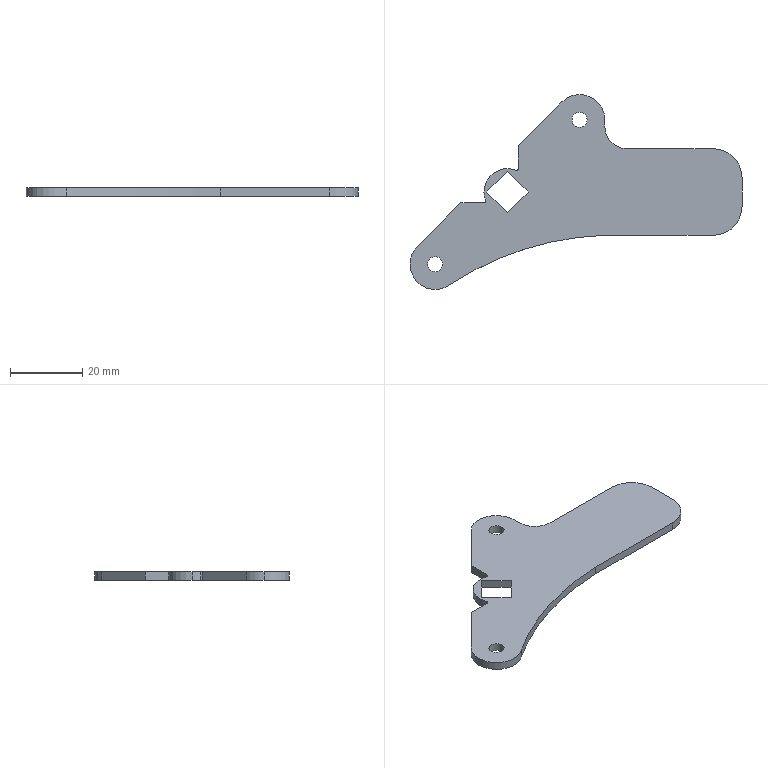Part | SolidWorks | features BaseBody 1 | 1 solid | 29 faces | box 92 x 54 x 2.3 mm | volume 5122 mm3 | cylinder 15 | plane 14 | commonest cylinder face diameters 4.2 x4 14 x3 1 x2 13 x2 16 x2 12 x1
STEP:
#1=CARTESIAN_POINT('',(-6.5,0.,2.3));
#2=VERTEX_POINT('',#1);
#3=CARTESIAN_POINT('',(-6.071,-2.321,2.3));
#4=VERTEX_POINT('',#3);
#5=CARTESIAN_POINT('',(0.,0.,2.3));
#6=DIRECTION('',(0.,0.,1.));
#7=DIRECTION('',(0.3571,0.934,0.));
#8=AXIS2_PLACEMENT_3D('',#5,#6,#7);
#9=CIRCLE('',#8,6.5);
#10=EDGE_CURVE('',#2,#4,#9,.T.);
#11=ORIENTED_EDGE('',*,*,#10,.F.);
#12=CARTESIAN_POINT('',(-6.5,0.,0.));
#13=VERTEX_POINT('',#12);
#14=CARTESIAN_POINT('',(-6.5,0.,2.3));
#15=DIRECTION('',(0.,0.,-1.));
#16=VECTOR('',#15,1000.);
#17=LINE('',#14,#16);
#18=EDGE_CURVE('',#2,#13,#17,.T.);
#19=ORIENTED_EDGE('',*,*,#18,.T.);
#20=CARTESIAN_POINT('',(-6.071,-2.321,0.));
#21=VERTEX_POINT('',#20);
#22=CARTESIAN_POINT('',(0.,0.,0.));
#23=DIRECTION('',(0.,0.,1.));
#24=DIRECTION('',(0.3571,0.934,0.));
#25=AXIS2_PLACEMENT_3D('',#22,#23,#24);
#26=CIRCLE('',#25,6.5);
#27=EDGE_CURVE('',#13,#21,#26,.T.);
#28=ORIENTED_EDGE('',*,*,#27,.T.);
#29=CARTESIAN_POINT('',(-6.071,-2.321,2.3));
#30=DIRECTION('',(0.,0.,-1.));
#31=VECTOR('',#30,1000.);
#32=LINE('',#29,#31);
#33=EDGE_CURVE('',#4,#21,#32,.T.);
#34=ORIENTED_EDGE('',*,*,#33,.F.);
#35=EDGE_LOOP('',(#11,#19,#28,#34));
#36=FACE_OUTER_BOUND('',#35,.T.);
#37=CARTESIAN_POINT('',(0.,0.,2.3));
#38=DIRECTION('',(0.,0.,-1.));
#39=DIRECTION('',(-1.,0.,0.));
#40=AXIS2_PLACEMENT_3D('',#37,#38,#39);
#41=CYLINDRICAL_SURFACE('',#40,6.5);
#42=ADVANCED_FACE('',(#36),#41,.T.);
#43=CARTESIAN_POINT('',(17.9,20.,2.3));
#44=VERTEX_POINT('',#43);
#45=CARTESIAN_POINT('',(22.1,20.,2.3));
#46=VERTEX_POINT('',#45);
#47=CARTESIAN_POINT('',(20.,20.,2.3));
#48=DIRECTION('',(0.,0.,1.));
#49=DIRECTION('',(1.,0.,0.));
#50=AXIS2_PLACEMENT_3D('',#47,#48,#49);
#51=CIRCLE('',#50,2.1);
#52=EDGE_CURVE('',#44,#46,#51,.T.);
#53=ORIENTED_EDGE('',*,*,#52,.T.);
#54=CARTESIAN_POINT('',(22.1,20.,0.));
#55=VERTEX_POINT('',#54);
#56=CARTESIAN_POINT('',(22.1,20.,2.3));
#57=DIRECTION('',(0.,0.,-1.));
#58=VECTOR('',#57,1000.);
#59=LINE('',#56,#58);
#60=EDGE_CURVE('',#46,#55,#59,.T.);
#61=ORIENTED_EDGE('',*,*,#60,.T.);
#62=CARTESIAN_POINT('',(17.9,20.,0.));
#63=VERTEX_POINT('',#62);
#64=CARTESIAN_POINT('',(20.,20.,0.));
#65=DIRECTION('',(0.,0.,1.));
#66=DIRECTION('',(1.,0.,0.));
#67=AXIS2_PLACEMENT_3D('',#64,#65,#66);
#68=CIRCLE('',#67,2.1);
#69=EDGE_CURVE('',#63,#55,#68,.T.);
#70=ORIENTED_EDGE('',*,*,#69,.F.);
#71=CARTESIAN_POINT('',(17.9,20.,2.3));
#72=DIRECTION('',(0.,0.,-1.));
#73=VECTOR('',#72,1000.);
#74=LINE('',#71,#73);
#75=EDGE_CURVE('',#44,#63,#74,.T.);
#76=ORIENTED_EDGE('',*,*,#75,.F.);
#77=EDGE_LOOP('',(#53,#61,#70,#76));
#78=FACE_OUTER_BOUND('',#77,.T.);
#79=CARTESIAN_POINT('',(20.,20.,2.3));
#80=DIRECTION('',(0.,0.,-1.));
#81=DIRECTION('',(-1.,0.,0.));
#82=AXIS2_PLACEMENT_3D('',#79,#80,#81);
#83=CYLINDRICAL_SURFACE('',#82,2.1);
#84=ADVANCED_FACE('',(#78),#83,.F.);
#85=CARTESIAN_POINT('',(-22.1,-20.,2.3));
#86=VERTEX_POINT('',#85);
#87=CARTESIAN_POINT('',(-17.9,-20.,2.3));
#88=VERTEX_POINT('',#87);
#89=CARTESIAN_POINT('',(-20.,-20.,2.3));
#90=DIRECTION('',(0.,0.,1.));
#91=DIRECTION('',(1.,0.,0.));
#92=AXIS2_PLACEMENT_3D('',#89,#90,#91);
#93=CIRCLE('',#92,2.1);
#94=EDGE_CURVE('',#86,#88,#93,.T.);
#95=ORIENTED_EDGE('',*,*,#94,.T.);
#96=CARTESIAN_POINT('',(-17.9,-20.,0.));
#97=VERTEX_POINT('',#96);
#98=CARTESIAN_POINT('',(-17.9,-20.,2.3));
#99=DIRECTION('',(0.,0.,-1.));
#100=VECTOR('',#99,1000.);
#101=LINE('',#98,#100);
#102=EDGE_CURVE('',#88,#97,#101,.T.);
#103=ORIENTED_EDGE('',*,*,#102,.T.);
#104=CARTESIAN_POINT('',(-22.1,-20.,0.));
#105=VERTEX_POINT('',#104);
#106=CARTESIAN_POINT('',(-20.,-20.,0.));
#107=DIRECTION('',(0.,0.,1.));
#108=DIRECTION('',(1.,0.,0.));
#109=AXIS2_PLACEMENT_3D('',#106,#107,#108);
#110=CIRCLE('',#109,2.1);
#111=EDGE_CURVE('',#105,#97,#110,.T.);
#112=ORIENTED_EDGE('',*,*,#111,.F.);
#113=CARTESIAN_POINT('',(-22.1,-20.,2.3));
#114=DIRECTION('',(0.,0.,-1.));
#115=VECTOR('',#114,1000.);
#116=LINE('',#113,#115);
#117=EDGE_CURVE('',#86,#105,#116,.T.);
#118=ORIENTED_EDGE('',*,*,#117,.F.);
#119=EDGE_LOOP('',(#95,#103,#112,#118));
#120=FACE_OUTER_BOUND('',#119,.T.);
#121=CARTESIAN_POINT('',(-20.,-20.,2.3));
#122=DIRECTION('',(0.,0.,-1.));
#123=DIRECTION('',(-1.,0.,0.));
#124=AXIS2_PLACEMENT_3D('',#121,#122,#123);
#125=CYLINDRICAL_SURFACE('',#124,2.1);
#126=ADVANCED_FACE('',(#120),#125,.F.);
#127=CARTESIAN_POINT('',(-27.,-20.,2.3));
#128=VERTEX_POINT('',#127);
#129=CARTESIAN_POINT('',(-15.783,-25.588,2.3));
#130=VERTEX_POINT('',#129);
#131=CARTESIAN_POINT('',(-20.,-20.,2.3));
#132=DIRECTION('',(0.,0.,1.));
#133=DIRECTION('',(-0.7071,0.7071,0.));
#134=AXIS2_PLACEMENT_3D('',#131,#132,#133);
#135=CIRCLE('',#134,7.);
#136=EDGE_CURVE('',#128,#130,#135,.T.);
#137=ORIENTED_EDGE('',*,*,#136,.F.);
#138=CARTESIAN_POINT('',(-27.,-20.,0.));
#139=VERTEX_POINT('',#138);
#140=CARTESIAN_POINT('',(-27.,-20.,2.3));
#141=DIRECTION('',(0.,0.,-1.));
#142=VECTOR('',#141,1000.);
#143=LINE('',#140,#142);
#144=EDGE_CURVE('',#128,#139,#143,.T.);
#145=ORIENTED_EDGE('',*,*,#144,.T.);
#146=CARTESIAN_POINT('',(-15.783,-25.588,0.));
#147=VERTEX_POINT('',#146);
#148=CARTESIAN_POINT('',(-20.,-20.,0.));
#149=DIRECTION('',(0.,0.,1.));
#150=DIRECTION('',(-0.7071,0.7071,0.));
#151=AXIS2_PLACEMENT_3D('',#148,#149,#150);
#152=CIRCLE('',#151,7.);
#153=EDGE_CURVE('',#139,#147,#152,.T.);
#154=ORIENTED_EDGE('',*,*,#153,.T.);
#155=CARTESIAN_POINT('',(-15.783,-25.588,2.3));
#156=DIRECTION('',(0.,0.,-1.));
#157=VECTOR('',#156,1000.);
#158=LINE('',#155,#157);
#159=EDGE_CURVE('',#130,#147,#158,.T.);
#160=ORIENTED_EDGE('',*,*,#159,.F.);
#161=EDGE_LOOP('',(#137,#145,#154,#160));
#162=FACE_OUTER_BOUND('',#161,.T.);
#163=CARTESIAN_POINT('',(-20.,-20.,2.3));
#164=DIRECTION('',(0.,0.,-1.));
#165=DIRECTION('',(-1.,0.,0.));
#166=AXIS2_PLACEMENT_3D('',#163,#164,#165);
#167=CYLINDRICAL_SURFACE('',#166,7.);
#168=ADVANCED_FACE('',(#162),#167,.T.);
#169=CARTESIAN_POINT('',(-12.899,-3.,0.));
#170=VERTEX_POINT('',#169);
#171=CARTESIAN_POINT('',(-24.95,-15.05,0.));
#172=VERTEX_POINT('',#171);
#173=CARTESIAN_POINT('',(-12.899,-3.,0.));
#174=DIRECTION('',(-0.7071,-0.7071,0.));
#175=VECTOR('',#174,1000.);
#176=LINE('',#173,#175);
#177=EDGE_CURVE('',#170,#172,#176,.T.);
#178=ORIENTED_EDGE('',*,*,#177,.T.);
#179=CARTESIAN_POINT('',(-24.95,-15.05,2.3));
#180=VERTEX_POINT('',#179);
#181=CARTESIAN_POINT('',(-24.95,-15.05,2.3));
#182=DIRECTION('',(0.,0.,-1.));
#183=VECTOR('',#182,1000.);
#184=LINE('',#181,#183);
#185=EDGE_CURVE('',#180,#172,#184,.T.);
#186=ORIENTED_EDGE('',*,*,#185,.F.);
#187=CARTESIAN_POINT('',(-12.899,-3.,2.3));
#188=VERTEX_POINT('',#187);
#189=CARTESIAN_POINT('',(-12.899,-3.,2.3));
#190=DIRECTION('',(-0.7071,-0.7071,0.));
#191=VECTOR('',#190,1000.);
#192=LINE('',#189,#191);
#193=EDGE_CURVE('',#188,#180,#192,.T.);
#194=ORIENTED_EDGE('',*,*,#193,.F.);
#195=CARTESIAN_POINT('',(-12.899,-3.,2.3));
#196=DIRECTION('',(0.,0.,-1.));
#197=VECTOR('',#196,1000.);
#198=LINE('',#195,#197);
#199=EDGE_CURVE('',#188,#170,#198,.T.);
#200=ORIENTED_EDGE('',*,*,#199,.T.);
#201=EDGE_LOOP('',(#178,#186,#194,#200));
#202=FACE_OUTER_BOUND('',#201,.T.);
#203=CARTESIAN_POINT('',(-12.899,-3.,2.3));
#204=DIRECTION('',(0.7071,-0.7071,0.));
#205=DIRECTION('',(0.7071,0.7071,0.));
#206=AXIS2_PLACEMENT_3D('',#203,#204,#205);
#207=PLANE('',#206);
#208=ADVANCED_FACE('',(#202),#207,.F.);
#209=ORIENTED_EDGE('',*,*,#111,.T.);
#210=CARTESIAN_POINT('',(-20.,-20.,0.));
#211=DIRECTION('',(0.,0.,1.));
#212=DIRECTION('',(1.,0.,0.));
#213=AXIS2_PLACEMENT_3D('',#210,#211,#212);
#214=CIRCLE('',#213,2.1);
#215=EDGE_CURVE('',#97,#105,#214,.T.);
#216=ORIENTED_EDGE('',*,*,#215,.T.);
#217=EDGE_LOOP('',(#209,#216));
#218=FACE_BOUND('',#217,.T.);
#219=CARTESIAN_POINT('',(0.,5.728,0.));
#220=VERTEX_POINT('',#219);
#221=CARTESIAN_POINT('',(-5.728,0.,0.));
#222=VERTEX_POINT('',#221);
#223=CARTESIAN_POINT('',(0.,5.728,0.));
#224=DIRECTION('',(-0.7071,-0.7071,0.));
#225=VECTOR('',#224,1000.);
#226=LINE('',#223,#225);
#227=EDGE_CURVE('',#220,#222,#226,.T.);
#228=ORIENTED_EDGE('',*,*,#227,.T.);
#229=CARTESIAN_POINT('',(0.,-5.728,0.));
#230=VERTEX_POINT('',#229);
#231=CARTESIAN_POINT('',(-5.728,0.,0.));
#232=DIRECTION('',(0.7071,-0.7071,0.));
#233=VECTOR('',#232,1000.);
#234=LINE('',#231,#233);
#235=EDGE_CURVE('',#222,#230,#234,.T.);
#236=ORIENTED_EDGE('',*,*,#235,.T.);
#237=CARTESIAN_POINT('',(5.728,0.,0.));
#238=VERTEX_POINT('',#237);
#239=CARTESIAN_POINT('',(0.,-5.728,0.));
#240=DIRECTION('',(0.7071,0.7071,0.));
#241=VECTOR('',#240,1000.);
#242=LINE('',#239,#241);
#243=EDGE_CURVE('',#230,#238,#242,.T.);
#244=ORIENTED_EDGE('',*,*,#243,.T.);
#245=CARTESIAN_POINT('',(5.728,0.,0.));
#246=DIRECTION('',(-0.7071,0.7071,0.));
#247=VECTOR('',#246,1000.);
#248=LINE('',#245,#247);
#249=EDGE_CURVE('',#238,#220,#248,.T.);
#250=ORIENTED_EDGE('',*,*,#249,.T.);
#251=EDGE_LOOP('',(#228,#236,#244,#250));
#252=FACE_BOUND('',#251,.T.);
#253=ORIENTED_EDGE('',*,*,#69,.T.);
#254=CARTESIAN_POINT('',(20.,20.,0.));
#255=DIRECTION('',(0.,0.,1.));
#256=DIRECTION('',(1.,0.,0.));
#257=AXIS2_PLACEMENT_3D('',#254,#255,#256);
#258=CIRCLE('',#257,2.1);
#259=EDGE_CURVE('',#55,#63,#258,.T.);
#260=ORIENTED_EDGE('',*,*,#259,.T.);
#261=EDGE_LOOP('',(#253,#260));
#262=FACE_BOUND('',#261,.T.);
#263=ORIENTED_EDGE('',*,*,#177,.F.);
#264=CARTESIAN_POINT('',(-6.538,-3.,0.));
#265=VERTEX_POINT('',#264);
#266=CARTESIAN_POINT('',(-6.538,-3.,0.));
#267=DIRECTION('',(-1.,0.,0.));
#268=VECTOR('',#267,1000.);
#269=LINE('',#266,#268);
#270=EDGE_CURVE('',#265,#170,#269,.T.);
#271=ORIENTED_EDGE('',*,*,#270,.F.);
#272=CARTESIAN_POINT('',(-6.538,-2.5,0.));
#273=DIRECTION('',(0.,0.,1.));
#274=DIRECTION('',(0.,-1.,0.));
#275=AXIS2_PLACEMENT_3D('',#272,#273,#274);
#276=CIRCLE('',#275,0.5);
#277=EDGE_CURVE('',#265,#21,#276,.T.);
#278=ORIENTED_EDGE('',*,*,#277,.T.);
#279=ORIENTED_EDGE('',*,*,#27,.F.);
#280=CARTESIAN_POINT('',(2.321,6.071,0.));
#281=VERTEX_POINT('',#280);
#282=CARTESIAN_POINT('',(0.,0.,0.));
#283=DIRECTION('',(0.,0.,1.));
#284=DIRECTION('',(0.3571,0.934,0.));
#285=AXIS2_PLACEMENT_3D('',#282,#283,#284);
#286=CIRCLE('',#285,6.5);
#287=EDGE_CURVE('',#281,#13,#286,.T.);
#288=ORIENTED_EDGE('',*,*,#287,.F.);
#289=CARTESIAN_POINT('',(3.,6.538,0.));
#290=VERTEX_POINT('',#289);
#291=CARTESIAN_POINT('',(2.5,6.538,0.));
#292=DIRECTION('',(0.,0.,1.));
#293=DIRECTION('',(-0.3571,-0.934,0.));
#294=AXIS2_PLACEMENT_3D('',#291,#292,#293);
#295=CIRCLE('',#294,0.5);
#296=EDGE_CURVE('',#281,#290,#295,.T.);
#297=ORIENTED_EDGE('',*,*,#296,.T.);
#298=CARTESIAN_POINT('',(3.,12.899,0.));
#299=VERTEX_POINT('',#298);
#300=CARTESIAN_POINT('',(3.,12.899,0.));
#301=DIRECTION('',(0.,-1.,0.));
#302=VECTOR('',#301,1000.);
#303=LINE('',#300,#302);
#304=EDGE_CURVE('',#299,#290,#303,.T.);
#305=ORIENTED_EDGE('',*,*,#304,.F.);
#306=CARTESIAN_POINT('',(15.05,24.95,0.));
#307=VERTEX_POINT('',#306);
#308=CARTESIAN_POINT('',(15.05,24.95,0.));
#309=DIRECTION('',(-0.7071,-0.7071,0.));
#310=VECTOR('',#309,1000.);
#311=LINE('',#308,#310);
#312=EDGE_CURVE('',#307,#299,#311,.T.);
#313=ORIENTED_EDGE('',*,*,#312,.F.);
#314=CARTESIAN_POINT('',(27.,20.,0.));
#315=VERTEX_POINT('',#314);
#316=CARTESIAN_POINT('',(20.,20.,0.));
#317=DIRECTION('',(0.,0.,1.));
#318=DIRECTION('',(1.,0.,0.));
#319=AXIS2_PLACEMENT_3D('',#316,#317,#318);
#320=CIRCLE('',#319,7.);
#321=EDGE_CURVE('',#315,#307,#320,.T.);
#322=ORIENTED_EDGE('',*,*,#321,.F.);
#323=CARTESIAN_POINT('',(27.,18.,0.));
#324=VERTEX_POINT('',#323);
#325=CARTESIAN_POINT('',(27.,18.,0.));
#326=DIRECTION('',(0.,1.,0.));
#327=VECTOR('',#326,1000.);
#328=LINE('',#325,#327);
#329=EDGE_CURVE('',#324,#315,#328,.T.);
#330=ORIENTED_EDGE('',*,*,#329,.F.);
#331=CARTESIAN_POINT('',(33.,12.,0.));
#332=VERTEX_POINT('',#331);
#333=CARTESIAN_POINT('',(33.,18.,0.));
#334=DIRECTION('',(0.,0.,1.));
#335=DIRECTION('',(-1.,0.,0.));
#336=AXIS2_PLACEMENT_3D('',#333,#334,#335);
#337=CIRCLE('',#336,6.);
#338=EDGE_CURVE('',#324,#332,#337,.T.);
#339=ORIENTED_EDGE('',*,*,#338,.T.);
#340=CARTESIAN_POINT('',(57.,12.,0.));
#341=VERTEX_POINT('',#340);
#342=CARTESIAN_POINT('',(57.,12.,0.));
#343=DIRECTION('',(-1.,0.,0.));
#344=VECTOR('',#343,1000.);
#345=LINE('',#342,#344);
#346=EDGE_CURVE('',#341,#332,#345,.T.);
#347=ORIENTED_EDGE('',*,*,#346,.F.);
#348=CARTESIAN_POINT('',(65.,4.,0.));
#349=VERTEX_POINT('',#348);
#350=CARTESIAN_POINT('',(57.,4.,0.));
#351=DIRECTION('',(0.,0.,1.));
#352=DIRECTION('',(1.,0.,0.));
#353=AXIS2_PLACEMENT_3D('',#350,#351,#352);
#354=CIRCLE('',#353,8.);
#355=EDGE_CURVE('',#349,#341,#354,.T.);
#356=ORIENTED_EDGE('',*,*,#355,.F.);
#357=CARTESIAN_POINT('',(65.,-4.,0.));
#358=VERTEX_POINT('',#357);
#359=CARTESIAN_POINT('',(65.,-4.,0.));
#360=DIRECTION('',(0.,1.,0.));
#361=VECTOR('',#360,1000.);
#362=LINE('',#359,#361);
#363=EDGE_CURVE('',#358,#349,#362,.T.);
#364=ORIENTED_EDGE('',*,*,#363,.F.);
#365=CARTESIAN_POINT('',(57.,-12.,0.));
#366=VERTEX_POINT('',#365);
#367=CARTESIAN_POINT('',(57.,-4.,0.));
#368=DIRECTION('',(0.,0.,1.));
#369=DIRECTION('',(0.,-1.,0.));
#370=AXIS2_PLACEMENT_3D('',#367,#368,#369);
#371=CIRCLE('',#370,8.);
#372=EDGE_CURVE('',#366,#358,#371,.T.);
#373=ORIENTED_EDGE('',*,*,#372,.F.);
#374=CARTESIAN_POINT('',(26.919,-12.,0.));
#375=VERTEX_POINT('',#374);
#376=CARTESIAN_POINT('',(26.919,-12.,0.));
#377=DIRECTION('',(1.,0.,0.));
#378=VECTOR('',#377,1000.);
#379=LINE('',#376,#378);
#380=EDGE_CURVE('',#375,#366,#379,.T.);
#381=ORIENTED_EDGE('',*,*,#380,.F.);
#382=CARTESIAN_POINT('',(29.8,-94.95,0.));
#383=DIRECTION('',(0.,0.,1.));
#384=DIRECTION('',(-0.03471,0.9994,0.));
#385=AXIS2_PLACEMENT_3D('',#382,#383,#384);
#386=CIRCLE('',#385,83.);
#387=EDGE_CURVE('',#375,#147,#386,.T.);
#388=ORIENTED_EDGE('',*,*,#387,.T.);
#389=ORIENTED_EDGE('',*,*,#153,.F.);
#390=CARTESIAN_POINT('',(-20.,-20.,0.));
#391=DIRECTION('',(0.,0.,1.));
#392=DIRECTION('',(-0.7071,0.7071,0.));
#393=AXIS2_PLACEMENT_3D('',#390,#391,#392);
#394=CIRCLE('',#393,7.);
#395=EDGE_CURVE('',#172,#139,#394,.T.);
#396=ORIENTED_EDGE('',*,*,#395,.F.);
#397=EDGE_LOOP('',(#263,#271,#278,#279,#288,#297,#305,#313,#322,#330,#339,#347,#356,#364,#373,#381,#388,#389,#396));
#398=FACE_OUTER_BOUND('',#397,.T.);
#399=CARTESIAN_POINT('',(-20.,-20.,0.));
#400=DIRECTION('',(0.,0.,1.));
#401=DIRECTION('',(1.,0.,0.));
#402=AXIS2_PLACEMENT_3D('',#399,#400,#401);
#403=PLANE('',#402);
#404=ADVANCED_FACE('',(#218,#252,#262,#398),#403,.F.);
#405=ORIENTED_EDGE('',*,*,#144,.F.);
#406=CARTESIAN_POINT('',(-20.,-20.,2.3));
#407=DIRECTION('',(0.,0.,1.));
#408=DIRECTION('',(-0.7071,0.7071,0.));
#409=AXIS2_PLACEMENT_3D('',#406,#407,#408);
#410=CIRCLE('',#409,7.);
#411=EDGE_CURVE('',#180,#128,#410,.T.);
#412=ORIENTED_EDGE('',*,*,#411,.F.);
#413=ORIENTED_EDGE('',*,*,#185,.T.);
#414=ORIENTED_EDGE('',*,*,#395,.T.);
#415=EDGE_LOOP('',(#405,#412,#413,#414));
#416=FACE_OUTER_BOUND('',#415,.T.);
#417=CARTESIAN_POINT('',(-20.,-20.,2.3));
#418=DIRECTION('',(0.,0.,-1.));
#419=DIRECTION('',(-1.,0.,0.));
#420=AXIS2_PLACEMENT_3D('',#417,#418,#419);
#421=CYLINDRICAL_SURFACE('',#420,7.);
#422=ADVANCED_FACE('',(#416),#421,.T.);
#423=ORIENTED_EDGE('',*,*,#94,.F.);
#424=CARTESIAN_POINT('',(-20.,-20.,2.3));
#425=DIRECTION('',(0.,0.,1.));
#426=DIRECTION('',(1.,0.,0.));
#427=AXIS2_PLACEMENT_3D('',#424,#425,#426);
#428=CIRCLE('',#427,2.1);
#429=EDGE_CURVE('',#88,#86,#428,.T.);
#430=ORIENTED_EDGE('',*,*,#429,.F.);
#431=EDGE_LOOP('',(#423,#430));
#432=FACE_BOUND('',#431,.T.);
#433=CARTESIAN_POINT('',(0.,5.728,2.3));
#434=VERTEX_POINT('',#433);
#435=CARTESIAN_POINT('',(-5.728,0.,2.3));
#436=VERTEX_POINT('',#435);
#437=CARTESIAN_POINT('',(0.,5.728,2.3));
#438=DIRECTION('',(-0.7071,-0.7071,0.));
#439=VECTOR('',#438,1000.);
#440=LINE('',#437,#439);
#441=EDGE_CURVE('',#434,#436,#440,.T.);
#442=ORIENTED_EDGE('',*,*,#441,.F.);
#443=CARTESIAN_POINT('',(5.728,0.,2.3));
#444=VERTEX_POINT('',#443);
#445=CARTESIAN_POINT('',(5.728,0.,2.3));
#446=DIRECTION('',(-0.7071,0.7071,0.));
#447=VECTOR('',#446,1000.);
#448=LINE('',#445,#447);
#449=EDGE_CURVE('',#444,#434,#448,.T.);
#450=ORIENTED_EDGE('',*,*,#449,.F.);
#451=CARTESIAN_POINT('',(0.,-5.728,2.3));
#452=VERTEX_POINT('',#451);
#453=CARTESIAN_POINT('',(0.,-5.728,2.3));
#454=DIRECTION('',(0.7071,0.7071,0.));
#455=VECTOR('',#454,1000.);
#456=LINE('',#453,#455);
#457=EDGE_CURVE('',#452,#444,#456,.T.);
#458=ORIENTED_EDGE('',*,*,#457,.F.);
#459=CARTESIAN_POINT('',(-5.728,0.,2.3));
#460=DIRECTION('',(0.7071,-0.7071,0.));
#461=VECTOR('',#460,1000.);
#462=LINE('',#459,#461);
#463=EDGE_CURVE('',#436,#452,#462,.T.);
#464=ORIENTED_EDGE('',*,*,#463,.F.);
#465=EDGE_LOOP('',(#442,#450,#458,#464));
#466=FACE_BOUND('',#465,.T.);
#467=ORIENTED_EDGE('',*,*,#52,.F.);
#468=CARTESIAN_POINT('',(20.,20.,2.3));
#469=DIRECTION('',(0.,0.,1.));
#470=DIRECTION('',(1.,0.,0.));
#471=AXIS2_PLACEMENT_3D('',#468,#469,#470);
#472=CIRCLE('',#471,2.1);
#473=EDGE_CURVE('',#46,#44,#472,.T.);
#474=ORIENTED_EDGE('',*,*,#473,.F.);
#475=EDGE_LOOP('',(#467,#474));
#476=FACE_BOUND('',#475,.T.);
#477=ORIENTED_EDGE('',*,*,#193,.T.);
#478=ORIENTED_EDGE('',*,*,#411,.T.);
#479=ORIENTED_EDGE('',*,*,#136,.T.);
#480=CARTESIAN_POINT('',(26.919,-12.,2.3));
#481=VERTEX_POINT('',#480);
#482=CARTESIAN_POINT('',(29.8,-94.95,2.3));
#483=DIRECTION('',(0.,0.,1.));
#484=DIRECTION('',(-0.03471,0.9994,0.));
#485=AXIS2_PLACEMENT_3D('',#482,#483,#484);
#486=CIRCLE('',#485,83.);
#487=EDGE_CURVE('',#481,#130,#486,.T.);
#488=ORIENTED_EDGE('',*,*,#487,.F.);
#489=CARTESIAN_POINT('',(57.,-12.,2.3));
#490=VERTEX_POINT('',#489);
#491=CARTESIAN_POINT('',(26.919,-12.,2.3));
#492=DIRECTION('',(1.,0.,0.));
#493=VECTOR('',#492,1000.);
#494=LINE('',#491,#493);
#495=EDGE_CURVE('',#481,#490,#494,.T.);
#496=ORIENTED_EDGE('',*,*,#495,.T.);
#497=CARTESIAN_POINT('',(65.,-4.,2.3));
#498=VERTEX_POINT('',#497);
#499=CARTESIAN_POINT('',(57.,-4.,2.3));
#500=DIRECTION('',(0.,0.,1.));
#501=DIRECTION('',(0.,-1.,0.));
#502=AXIS2_PLACEMENT_3D('',#499,#500,#501);
#503=CIRCLE('',#502,8.);
#504=EDGE_CURVE('',#490,#498,#503,.T.);
#505=ORIENTED_EDGE('',*,*,#504,.T.);
#506=CARTESIAN_POINT('',(65.,4.,2.3));
#507=VERTEX_POINT('',#506);
#508=CARTESIAN_POINT('',(65.,-4.,2.3));
#509=DIRECTION('',(0.,1.,0.));
#510=VECTOR('',#509,1000.);
#511=LINE('',#508,#510);
#512=EDGE_CURVE('',#498,#507,#511,.T.);
#513=ORIENTED_EDGE('',*,*,#512,.T.);
#514=CARTESIAN_POINT('',(57.,12.,2.3));
#515=VERTEX_POINT('',#514);
#516=CARTESIAN_POINT('',(57.,4.,2.3));
#517=DIRECTION('',(0.,0.,1.));
#518=DIRECTION('',(1.,0.,0.));
#519=AXIS2_PLACEMENT_3D('',#516,#517,#518);
#520=CIRCLE('',#519,8.);
#521=EDGE_CURVE('',#507,#515,#520,.T.);
#522=ORIENTED_EDGE('',*,*,#521,.T.);
#523=CARTESIAN_POINT('',(33.,12.,2.3));
#524=VERTEX_POINT('',#523);
#525=CARTESIAN_POINT('',(57.,12.,2.3));
#526=DIRECTION('',(-1.,0.,0.));
#527=VECTOR('',#526,1000.);
#528=LINE('',#525,#527);
#529=EDGE_CURVE('',#515,#524,#528,.T.);
#530=ORIENTED_EDGE('',*,*,#529,.T.);
#531=CARTESIAN_POINT('',(27.,18.,2.3));
#532=VERTEX_POINT('',#531);
#533=CARTESIAN_POINT('',(33.,18.,2.3));
#534=DIRECTION('',(0.,0.,1.));
#535=DIRECTION('',(-1.,0.,0.));
#536=AXIS2_PLACEMENT_3D('',#533,#534,#535);
#537=CIRCLE('',#536,6.);
#538=EDGE_CURVE('',#532,#524,#537,.T.);
#539=ORIENTED_EDGE('',*,*,#538,.F.);
#540=CARTESIAN_POINT('',(27.,20.,2.3));
#541=VERTEX_POINT('',#540);
#542=CARTESIAN_POINT('',(27.,18.,2.3));
#543=DIRECTION('',(0.,1.,0.));
#544=VECTOR('',#543,1000.);
#545=LINE('',#542,#544);
#546=EDGE_CURVE('',#532,#541,#545,.T.);
#547=ORIENTED_EDGE('',*,*,#546,.T.);
#548=CARTESIAN_POINT('',(15.05,24.95,2.3));
#549=VERTEX_POINT('',#548);
#550=CARTESIAN_POINT('',(20.,20.,2.3));
#551=DIRECTION('',(0.,0.,1.));
#552=DIRECTION('',(1.,0.,0.));
#553=AXIS2_PLACEMENT_3D('',#550,#551,#552);
#554=CIRCLE('',#553,7.);
#555=EDGE_CURVE('',#541,#549,#554,.T.);
#556=ORIENTED_EDGE('',*,*,#555,.T.);
#557=CARTESIAN_POINT('',(3.,12.899,2.3));
#558=VERTEX_POINT('',#557);
#559=CARTESIAN_POINT('',(15.05,24.95,2.3));
#560=DIRECTION('',(-0.7071,-0.7071,0.));
#561=VECTOR('',#560,1000.);
#562=LINE('',#559,#561);
#563=EDGE_CURVE('',#549,#558,#562,.T.);
#564=ORIENTED_EDGE('',*,*,#563,.T.);
#565=CARTESIAN_POINT('',(3.,6.538,2.3));
#566=VERTEX_POINT('',#565);
#567=CARTESIAN_POINT('',(3.,12.899,2.3));
#568=DIRECTION('',(0.,-1.,0.));
#569=VECTOR('',#568,1000.);
#570=LINE('',#567,#569);
#571=EDGE_CURVE('',#558,#566,#570,.T.);
#572=ORIENTED_EDGE('',*,*,#571,.T.);
#573=CARTESIAN_POINT('',(2.321,6.071,2.3));
#574=VERTEX_POINT('',#573);
#575=CARTESIAN_POINT('',(2.5,6.538,2.3));
#576=DIRECTION('',(0.,0.,1.));
#577=DIRECTION('',(-0.3571,-0.934,0.));
#578=AXIS2_PLACEMENT_3D('',#575,#576,#577);
#579=CIRCLE('',#578,0.5);
#580=EDGE_CURVE('',#574,#566,#579,.T.);
#581=ORIENTED_EDGE('',*,*,#580,.F.);
#582=CARTESIAN_POINT('',(0.,0.,2.3));
#583=DIRECTION('',(0.,0.,1.));
#584=DIRECTION('',(0.3571,0.934,0.));
#585=AXIS2_PLACEMENT_3D('',#582,#583,#584);
#586=CIRCLE('',#585,6.5);
#587=EDGE_CURVE('',#574,#2,#586,.T.);
#588=ORIENTED_EDGE('',*,*,#587,.T.);
#589=ORIENTED_EDGE('',*,*,#10,.T.);
#590=CARTESIAN_POINT('',(-6.538,-3.,2.3));
#591=VERTEX_POINT('',#590);
#592=CARTESIAN_POINT('',(-6.538,-2.5,2.3));
#593=DIRECTION('',(0.,0.,1.));
#594=DIRECTION('',(0.,-1.,0.));
#595=AXIS2_PLACEMENT_3D('',#592,#593,#594);
#596=CIRCLE('',#595,0.5);
#597=EDGE_CURVE('',#591,#4,#596,.T.);
#598=ORIENTED_EDGE('',*,*,#597,.F.);
#599=CARTESIAN_POINT('',(-6.538,-3.,2.3));
#600=DIRECTION('',(-1.,0.,0.));
#601=VECTOR('',#600,1000.);
#602=LINE('',#599,#601);
#603=EDGE_CURVE('',#591,#188,#602,.T.);
#604=ORIENTED_EDGE('',*,*,#603,.T.);
#605=EDGE_LOOP('',(#477,#478,#479,#488,#496,#505,#513,#522,#530,#539,#547,#556,#564,#572,#581,#588,#589,#598,#604));
#606=FACE_OUTER_BOUND('',#605,.T.);
#607=CARTESIAN_POINT('',(-20.,-20.,2.3));
#608=DIRECTION('',(0.,0.,1.));
#609=DIRECTION('',(1.,0.,0.));
#610=AXIS2_PLACEMENT_3D('',#607,#608,#609);
#611=PLANE('',#610);
#612=ADVANCED_FACE('',(#432,#466,#476,#606),#611,.T.);
#613=ORIENTED_EDGE('',*,*,#270,.T.);
#614=ORIENTED_EDGE('',*,*,#199,.F.);
#615=ORIENTED_EDGE('',*,*,#603,.F.);
#616=CARTESIAN_POINT('',(-6.538,-3.,2.3));
#617=DIRECTION('',(0.,0.,-1.));
#618=VECTOR('',#617,1000.);
#619=LINE('',#616,#618);
#620=EDGE_CURVE('',#591,#265,#619,.T.);
#621=ORIENTED_EDGE('',*,*,#620,.T.);
#622=EDGE_LOOP('',(#613,#614,#615,#621));
#623=FACE_OUTER_BOUND('',#622,.T.);
#624=CARTESIAN_POINT('',(-6.538,-3.,2.3));
#625=DIRECTION('',(0.,-1.,0.));
#626=DIRECTION('',(0.,0.,-1.));
#627=AXIS2_PLACEMENT_3D('',#624,#625,#626);
#628=PLANE('',#627);
#629=ADVANCED_FACE('',(#623),#628,.F.);
#630=ORIENTED_EDGE('',*,*,#102,.F.);
#631=ORIENTED_EDGE('',*,*,#429,.T.);
#632=ORIENTED_EDGE('',*,*,#117,.T.);
#633=ORIENTED_EDGE('',*,*,#215,.F.);
#634=EDGE_LOOP('',(#630,#631,#632,#633));
#635=FACE_OUTER_BOUND('',#634,.T.);
#636=CARTESIAN_POINT('',(-20.,-20.,2.3));
#637=DIRECTION('',(0.,0.,-1.));
#638=DIRECTION('',(-1.,0.,0.));
#639=AXIS2_PLACEMENT_3D('',#636,#637,#638);
#640=CYLINDRICAL_SURFACE('',#639,2.1);
#641=ADVANCED_FACE('',(#635),#640,.F.);
#642=ORIENTED_EDGE('',*,*,#227,.F.);
#643=CARTESIAN_POINT('',(0.,5.728,2.3));
#644=DIRECTION('',(0.,0.,-1.));
#645=VECTOR('',#644,1000.);
#646=LINE('',#643,#645);
#647=EDGE_CURVE('',#434,#220,#646,.T.);
#648=ORIENTED_EDGE('',*,*,#647,.F.);
#649=ORIENTED_EDGE('',*,*,#441,.T.);
#650=CARTESIAN_POINT('',(-5.728,0.,2.3));
#651=DIRECTION('',(0.,0.,-1.));
#652=VECTOR('',#651,1000.);
#653=LINE('',#650,#652);
#654=EDGE_CURVE('',#436,#222,#653,.T.);
#655=ORIENTED_EDGE('',*,*,#654,.T.);
#656=EDGE_LOOP('',(#642,#648,#649,#655));
#657=FACE_OUTER_BOUND('',#656,.T.);
#658=CARTESIAN_POINT('',(0.,5.728,2.3));
#659=DIRECTION('',(0.7071,-0.7071,0.));
#660=DIRECTION('',(0.7071,0.7071,0.));
#661=AXIS2_PLACEMENT_3D('',#658,#659,#660);
#662=PLANE('',#661);
#663=ADVANCED_FACE('',(#657),#662,.T.);
#664=ORIENTED_EDGE('',*,*,#235,.F.);
#665=ORIENTED_EDGE('',*,*,#654,.F.);
#666=ORIENTED_EDGE('',*,*,#463,.T.);
#667=CARTESIAN_POINT('',(0.,-5.728,2.3));
#668=DIRECTION('',(0.,0.,-1.));
#669=VECTOR('',#668,1000.);
#670=LINE('',#667,#669);
#671=EDGE_CURVE('',#452,#230,#670,.T.);
#672=ORIENTED_EDGE('',*,*,#671,.T.);
#673=EDGE_LOOP('',(#664,#665,#666,#672));
#674=FACE_OUTER_BOUND('',#673,.T.);
#675=CARTESIAN_POINT('',(-5.728,0.,2.3));
#676=DIRECTION('',(0.7071,0.7071,0.));
#677=DIRECTION('',(-0.7071,0.7071,0.));
#678=AXIS2_PLACEMENT_3D('',#675,#676,#677);
#679=PLANE('',#678);
#680=ADVANCED_FACE('',(#674),#679,.T.);
#681=ORIENTED_EDGE('',*,*,#243,.F.);
#682=ORIENTED_EDGE('',*,*,#671,.F.);
#683=ORIENTED_EDGE('',*,*,#457,.T.);
#684=CARTESIAN_POINT('',(5.728,0.,2.3));
#685=DIRECTION('',(0.,0.,-1.));
#686=VECTOR('',#685,1000.);
#687=LINE('',#684,#686);
#688=EDGE_CURVE('',#444,#238,#687,.T.);
#689=ORIENTED_EDGE('',*,*,#688,.T.);
#690=EDGE_LOOP('',(#681,#682,#683,#689));
#691=FACE_OUTER_BOUND('',#690,.T.);
#692=CARTESIAN_POINT('',(0.,-5.728,2.3));
#693=DIRECTION('',(-0.7071,0.7071,0.));
#694=DIRECTION('',(-0.7071,-0.7071,0.));
#695=AXIS2_PLACEMENT_3D('',#692,#693,#694);
#696=PLANE('',#695);
#697=ADVANCED_FACE('',(#691),#696,.T.);
#698=ORIENTED_EDGE('',*,*,#249,.F.);
#699=ORIENTED_EDGE('',*,*,#688,.F.);
#700=ORIENTED_EDGE('',*,*,#449,.T.);
#701=ORIENTED_EDGE('',*,*,#647,.T.);
#702=EDGE_LOOP('',(#698,#699,#700,#701));
#703=FACE_OUTER_BOUND('',#702,.T.);
#704=CARTESIAN_POINT('',(5.728,0.,2.3));
#705=DIRECTION('',(-0.7071,-0.7071,0.));
#706=DIRECTION('',(0.7071,-0.7071,0.));
#707=AXIS2_PLACEMENT_3D('',#704,#705,#706);
#708=PLANE('',#707);
#709=ADVANCED_FACE('',(#703),#708,.T.);
#710=ORIENTED_EDGE('',*,*,#60,.F.);
#711=ORIENTED_EDGE('',*,*,#473,.T.);
#712=ORIENTED_EDGE('',*,*,#75,.T.);
#713=ORIENTED_EDGE('',*,*,#259,.F.);
#714=EDGE_LOOP('',(#710,#711,#712,#713));
#715=FACE_OUTER_BOUND('',#714,.T.);
#716=CARTESIAN_POINT('',(20.,20.,2.3));
#717=DIRECTION('',(0.,0.,-1.));
#718=DIRECTION('',(-1.,0.,0.));
#719=AXIS2_PLACEMENT_3D('',#716,#717,#718);
#720=CYLINDRICAL_SURFACE('',#719,2.1);
#721=ADVANCED_FACE('',(#715),#720,.F.);
#722=ORIENTED_EDGE('',*,*,#277,.F.);
#723=ORIENTED_EDGE('',*,*,#620,.F.);
#724=ORIENTED_EDGE('',*,*,#597,.T.);
#725=ORIENTED_EDGE('',*,*,#33,.T.);
#726=EDGE_LOOP('',(#722,#723,#724,#725));
#727=FACE_OUTER_BOUND('',#726,.T.);
#728=CARTESIAN_POINT('',(-6.538,-2.5,2.3));
#729=DIRECTION('',(0.,0.,-1.));
#730=DIRECTION('',(-1.,0.,0.));
#731=AXIS2_PLACEMENT_3D('',#728,#729,#730);
#732=CYLINDRICAL_SURFACE('',#731,0.5);
#733=ADVANCED_FACE('',(#727),#732,.F.);
#734=ORIENTED_EDGE('',*,*,#18,.F.);
#735=ORIENTED_EDGE('',*,*,#587,.F.);
#736=CARTESIAN_POINT('',(2.321,6.071,2.3));
#737=DIRECTION('',(0.,0.,-1.));
#738=VECTOR('',#737,1000.);
#739=LINE('',#736,#738);
#740=EDGE_CURVE('',#574,#281,#739,.T.);
#741=ORIENTED_EDGE('',*,*,#740,.T.);
#742=ORIENTED_EDGE('',*,*,#287,.T.);
#743=EDGE_LOOP('',(#734,#735,#741,#742));
#744=FACE_OUTER_BOUND('',#743,.T.);
#745=CARTESIAN_POINT('',(0.,0.,2.3));
#746=DIRECTION('',(0.,0.,-1.));
#747=DIRECTION('',(-1.,0.,0.));
#748=AXIS2_PLACEMENT_3D('',#745,#746,#747);
#749=CYLINDRICAL_SURFACE('',#748,6.5);
#750=ADVANCED_FACE('',(#744),#749,.T.);
#751=ORIENTED_EDGE('',*,*,#296,.F.);
#752=ORIENTED_EDGE('',*,*,#740,.F.);
#753=ORIENTED_EDGE('',*,*,#580,.T.);
#754=CARTESIAN_POINT('',(3.,6.538,2.3));
#755=DIRECTION('',(0.,0.,-1.));
#756=VECTOR('',#755,1000.);
#757=LINE('',#754,#756);
#758=EDGE_CURVE('',#566,#290,#757,.T.);
#759=ORIENTED_EDGE('',*,*,#758,.T.);
#760=EDGE_LOOP('',(#751,#752,#753,#759));
#761=FACE_OUTER_BOUND('',#760,.T.);
#762=CARTESIAN_POINT('',(2.5,6.538,2.3));
#763=DIRECTION('',(0.,0.,-1.));
#764=DIRECTION('',(-1.,0.,0.));
#765=AXIS2_PLACEMENT_3D('',#762,#763,#764);
#766=CYLINDRICAL_SURFACE('',#765,0.5);
#767=ADVANCED_FACE('',(#761),#766,.F.);
#768=ORIENTED_EDGE('',*,*,#304,.T.);
#769=ORIENTED_EDGE('',*,*,#758,.F.);
#770=ORIENTED_EDGE('',*,*,#571,.F.);
#771=CARTESIAN_POINT('',(3.,12.899,2.3));
#772=DIRECTION('',(0.,0.,-1.));
#773=VECTOR('',#772,1000.);
#774=LINE('',#771,#773);
#775=EDGE_CURVE('',#558,#299,#774,.T.);
#776=ORIENTED_EDGE('',*,*,#775,.T.);
#777=EDGE_LOOP('',(#768,#769,#770,#776));
#778=FACE_OUTER_BOUND('',#777,.T.);
#779=CARTESIAN_POINT('',(3.,12.899,2.3));
#780=DIRECTION('',(1.,0.,0.));
#781=DIRECTION('',(0.,0.,-1.));
#782=AXIS2_PLACEMENT_3D('',#779,#780,#781);
#783=PLANE('',#782);
#784=ADVANCED_FACE('',(#778),#783,.F.);
#785=ORIENTED_EDGE('',*,*,#312,.T.);
#786=ORIENTED_EDGE('',*,*,#775,.F.);
#787=ORIENTED_EDGE('',*,*,#563,.F.);
#788=CARTESIAN_POINT('',(15.05,24.95,2.3));
#789=DIRECTION('',(0.,0.,-1.));
#790=VECTOR('',#789,1000.);
#791=LINE('',#788,#790);
#792=EDGE_CURVE('',#549,#307,#791,.T.);
#793=ORIENTED_EDGE('',*,*,#792,.T.);
#794=EDGE_LOOP('',(#785,#786,#787,#793));
#795=FACE_OUTER_BOUND('',#794,.T.);
#796=CARTESIAN_POINT('',(15.05,24.95,2.3));
#797=DIRECTION('',(0.7071,-0.7071,0.));
#798=DIRECTION('',(0.7071,0.7071,0.));
#799=AXIS2_PLACEMENT_3D('',#796,#797,#798);
#800=PLANE('',#799);
#801=ADVANCED_FACE('',(#795),#800,.F.);
#802=ORIENTED_EDGE('',*,*,#321,.T.);
#803=ORIENTED_EDGE('',*,*,#792,.F.);
#804=ORIENTED_EDGE('',*,*,#555,.F.);
#805=CARTESIAN_POINT('',(27.,20.,2.3));
#806=DIRECTION('',(0.,0.,-1.));
#807=VECTOR('',#806,1000.);
#808=LINE('',#805,#807);
#809=EDGE_CURVE('',#541,#315,#808,.T.);
#810=ORIENTED_EDGE('',*,*,#809,.T.);
#811=EDGE_LOOP('',(#802,#803,#804,#810));
#812=FACE_OUTER_BOUND('',#811,.T.);
#813=CARTESIAN_POINT('',(20.,20.,2.3));
#814=DIRECTION('',(0.,0.,-1.));
#815=DIRECTION('',(-1.,0.,0.));
#816=AXIS2_PLACEMENT_3D('',#813,#814,#815);
#817=CYLINDRICAL_SURFACE('',#816,7.);
#818=ADVANCED_FACE('',(#812),#817,.T.);
#819=ORIENTED_EDGE('',*,*,#329,.T.);
#820=ORIENTED_EDGE('',*,*,#809,.F.);
#821=ORIENTED_EDGE('',*,*,#546,.F.);
#822=CARTESIAN_POINT('',(27.,18.,2.3));
#823=DIRECTION('',(0.,0.,-1.));
#824=VECTOR('',#823,1000.);
#825=LINE('',#822,#824);
#826=EDGE_CURVE('',#532,#324,#825,.T.);
#827=ORIENTED_EDGE('',*,*,#826,.T.);
#828=EDGE_LOOP('',(#819,#820,#821,#827));
#829=FACE_OUTER_BOUND('',#828,.T.);
#830=CARTESIAN_POINT('',(27.,18.,2.3));
#831=DIRECTION('',(-1.,0.,0.));
#832=DIRECTION('',(0.,0.,1.));
#833=AXIS2_PLACEMENT_3D('',#830,#831,#832);
#834=PLANE('',#833);
#835=ADVANCED_FACE('',(#829),#834,.F.);
#836=ORIENTED_EDGE('',*,*,#338,.F.);
#837=ORIENTED_EDGE('',*,*,#826,.F.);
#838=ORIENTED_EDGE('',*,*,#538,.T.);
#839=CARTESIAN_POINT('',(33.,12.,2.3));
#840=DIRECTION('',(0.,0.,-1.));
#841=VECTOR('',#840,1000.);
#842=LINE('',#839,#841);
#843=EDGE_CURVE('',#524,#332,#842,.T.);
#844=ORIENTED_EDGE('',*,*,#843,.T.);
#845=EDGE_LOOP('',(#836,#837,#838,#844));
#846=FACE_OUTER_BOUND('',#845,.T.);
#847=CARTESIAN_POINT('',(33.,18.,2.3));
#848=DIRECTION('',(0.,0.,-1.));
#849=DIRECTION('',(-1.,0.,0.));
#850=AXIS2_PLACEMENT_3D('',#847,#848,#849);
#851=CYLINDRICAL_SURFACE('',#850,6.);
#852=ADVANCED_FACE('',(#846),#851,.F.);
#853=ORIENTED_EDGE('',*,*,#346,.T.);
#854=ORIENTED_EDGE('',*,*,#843,.F.);
#855=ORIENTED_EDGE('',*,*,#529,.F.);
#856=CARTESIAN_POINT('',(57.,12.,2.3));
#857=DIRECTION('',(0.,0.,-1.));
#858=VECTOR('',#857,1000.);
#859=LINE('',#856,#858);
#860=EDGE_CURVE('',#515,#341,#859,.T.);
#861=ORIENTED_EDGE('',*,*,#860,.T.);
#862=EDGE_LOOP('',(#853,#854,#855,#861));
#863=FACE_OUTER_BOUND('',#862,.T.);
#864=CARTESIAN_POINT('',(57.,12.,2.3));
#865=DIRECTION('',(0.,-1.,0.));
#866=DIRECTION('',(0.,0.,-1.));
#867=AXIS2_PLACEMENT_3D('',#864,#865,#866);
#868=PLANE('',#867);
#869=ADVANCED_FACE('',(#863),#868,.F.);
#870=ORIENTED_EDGE('',*,*,#355,.T.);
#871=ORIENTED_EDGE('',*,*,#860,.F.);
#872=ORIENTED_EDGE('',*,*,#521,.F.);
#873=CARTESIAN_POINT('',(65.,4.,2.3));
#874=DIRECTION('',(0.,0.,-1.));
#875=VECTOR('',#874,1000.);
#876=LINE('',#873,#875);
#877=EDGE_CURVE('',#507,#349,#876,.T.);
#878=ORIENTED_EDGE('',*,*,#877,.T.);
#879=EDGE_LOOP('',(#870,#871,#872,#878));
#880=FACE_OUTER_BOUND('',#879,.T.);
#881=CARTESIAN_POINT('',(57.,4.,2.3));
#882=DIRECTION('',(0.,0.,-1.));
#883=DIRECTION('',(-1.,0.,0.));
#884=AXIS2_PLACEMENT_3D('',#881,#882,#883);
#885=CYLINDRICAL_SURFACE('',#884,8.);
#886=ADVANCED_FACE('',(#880),#885,.T.);
#887=ORIENTED_EDGE('',*,*,#363,.T.);
#888=ORIENTED_EDGE('',*,*,#877,.F.);
#889=ORIENTED_EDGE('',*,*,#512,.F.);
#890=CARTESIAN_POINT('',(65.,-4.,2.3));
#891=DIRECTION('',(0.,0.,-1.));
#892=VECTOR('',#891,1000.);
#893=LINE('',#890,#892);
#894=EDGE_CURVE('',#498,#358,#893,.T.);
#895=ORIENTED_EDGE('',*,*,#894,.T.);
#896=EDGE_LOOP('',(#887,#888,#889,#895));
#897=FACE_OUTER_BOUND('',#896,.T.);
#898=CARTESIAN_POINT('',(65.,-4.,2.3));
#899=DIRECTION('',(-1.,0.,0.));
#900=DIRECTION('',(0.,0.,1.));
#901=AXIS2_PLACEMENT_3D('',#898,#899,#900);
#902=PLANE('',#901);
#903=ADVANCED_FACE('',(#897),#902,.F.);
#904=ORIENTED_EDGE('',*,*,#372,.T.);
#905=ORIENTED_EDGE('',*,*,#894,.F.);
#906=ORIENTED_EDGE('',*,*,#504,.F.);
#907=CARTESIAN_POINT('',(57.,-12.,2.3));
#908=DIRECTION('',(0.,0.,-1.));
#909=VECTOR('',#908,1000.);
#910=LINE('',#907,#909);
#911=EDGE_CURVE('',#490,#366,#910,.T.);
#912=ORIENTED_EDGE('',*,*,#911,.T.);
#913=EDGE_LOOP('',(#904,#905,#906,#912));
#914=FACE_OUTER_BOUND('',#913,.T.);
#915=CARTESIAN_POINT('',(57.,-4.,2.3));
#916=DIRECTION('',(0.,0.,-1.));
#917=DIRECTION('',(-1.,0.,0.));
#918=AXIS2_PLACEMENT_3D('',#915,#916,#917);
#919=CYLINDRICAL_SURFACE('',#918,8.);
#920=ADVANCED_FACE('',(#914),#919,.T.);
#921=ORIENTED_EDGE('',*,*,#380,.T.);
#922=ORIENTED_EDGE('',*,*,#911,.F.);
#923=ORIENTED_EDGE('',*,*,#495,.F.);
#924=CARTESIAN_POINT('',(26.919,-12.,2.3));
#925=DIRECTION('',(0.,0.,-1.));
#926=VECTOR('',#925,1000.);
#927=LINE('',#924,#926);
#928=EDGE_CURVE('',#481,#375,#927,.T.);
#929=ORIENTED_EDGE('',*,*,#928,.T.);
#930=EDGE_LOOP('',(#921,#922,#923,#929));
#931=FACE_OUTER_BOUND('',#930,.T.);
#932=CARTESIAN_POINT('',(26.919,-12.,2.3));
#933=DIRECTION('',(0.,1.,0.));
#934=DIRECTION('',(0.,0.,1.));
#935=AXIS2_PLACEMENT_3D('',#932,#933,#934);
#936=PLANE('',#935);
#937=ADVANCED_FACE('',(#931),#936,.F.);
#938=ORIENTED_EDGE('',*,*,#387,.F.);
#939=ORIENTED_EDGE('',*,*,#928,.F.);
#940=ORIENTED_EDGE('',*,*,#487,.T.);
#941=ORIENTED_EDGE('',*,*,#159,.T.);
#942=EDGE_LOOP('',(#938,#939,#940,#941));
#943=FACE_OUTER_BOUND('',#942,.T.);
#944=CARTESIAN_POINT('',(29.8,-94.95,2.3));
#945=DIRECTION('',(0.,0.,-1.));
#946=DIRECTION('',(-1.,0.,0.));
#947=AXIS2_PLACEMENT_3D('',#944,#945,#946);
#948=CYLINDRICAL_SURFACE('',#947,83.);
#949=ADVANCED_FACE('',(#943),#948,.F.);
#950=CLOSED_SHELL('',(#42,#84,#126,#168,#208,#404,#422,#612,#629,#641,#663,#680,#697,#709,#721,#733,#750,#767,#784,#801,#818,#835,#852,#869,#886,#903,#920,#937,#949));
#951=MANIFOLD_SOLID_BREP('',#950);
#952=CARTESIAN_POINT('',(0.,0.,0.));
#953=DIRECTION('',(0.,0.,1.));
#954=DIRECTION('',(1.,0.,0.));
#955=AXIS2_PLACEMENT_3D('',#952,#953,#954);
#956=(LENGTH_UNIT()NAMED_UNIT(*)SI_UNIT(.MILLI.,.METRE.));
#957=UNCERTAINTY_MEASURE_WITH_UNIT(LENGTH_MEASURE(0.00001),#956,'','');
#958=(NAMED_UNIT(*)PLANE_ANGLE_UNIT()SI_UNIT($,.RADIAN.));
#959=(NAMED_UNIT(*)SI_UNIT($,.STERADIAN.)SOLID_ANGLE_UNIT());
#960=(GEOMETRIC_REPRESENTATION_CONTEXT(3)GLOBAL_UNCERTAINTY_ASSIGNED_CONTEXT((#957))GLOBAL_UNIT_ASSIGNED_CONTEXT((#956,#958,#959))REPRESENTATION_CONTEXT('',''));
#961=ADVANCED_BREP_SHAPE_REPRESENTATION('',(#951,#955),#960);